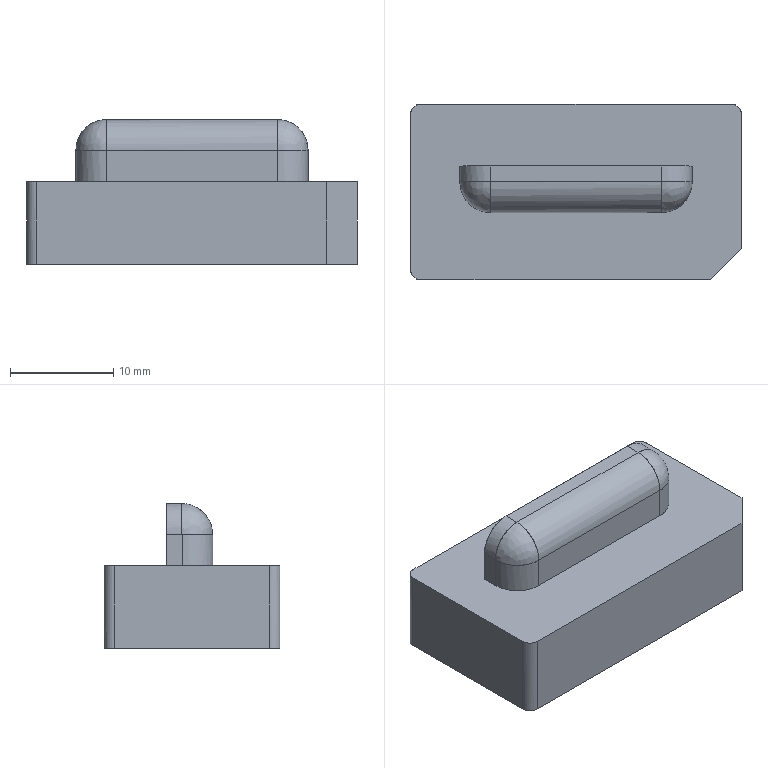NC program | PowerMill | posted with a generic post | part box 32 x 17 x 14 mm
Lines 1 to 1051 of 64476:
%
O0001
N104 ( POWERMILL CB  : 2026004.0)
N105 ( POST VER      : 2026.0.0.5161)
N106 ( OPTION FILE   : FANUC)
N107 ( OUTPUT WORKPLANE : WORLD)
N108 (  )
N109 ( TOOL LIST )
N110 (---------------------------------------)
N111 ( NO. | ID        | DIA.| TIP RAD|LENGTH)
N112 (---------------------------------------)
N113 (    1|D10C_1_1   |10.0 |  0.0   |69.44 )
N114 (    2|D4C_1_1    | 4.0 |  0.0   | 61.2 )
N115 (    3|D10_1_1    |10.0 |  0.0   |69.16 )
N116 (   22|R1.5_1_1   | 3.0 |  1.5   |59.88 )
N117 (   10|D3_1_1     | 3.0 |  0.0   |61.24 )
N118 (   13|TEXT_D4_1_1| 4.0 |  0.3   |61.24 )
N119 (---------------------------------------)
N120 (  )
N121 ( NUMBER OF TOOLPATHS: 10.0 )
N122 ( ESTIMATED PROGRAM DURATION: 0 HOURS 7 MIN 28 SEC)
N123 (  )
N124 G00 G21 G80 G40 G17
N125 G90
N126 G54
N127 G53 Z0.0
N128 (---------------)
N129 ( START TOOLPATH : 精公开粗01-扫面平行-D10C )
N130 (---------------)
N131 ( TOOL NO.    :1 )
N132 ( TOOL TYPE   : ENDMILL)
N133 ( TOOL ID     : D10C_1_1)
N134 ( TOOL DIA    : 10.0 LENGTH 69.44)
N135 T1
N136 M6
N137 S8000 M03
N138 G00 G90 X0.0 Y0.0
N139 G43 Z10.2 H1
N140
N141 G05 P10000 R4
N142 X23.78 Y11.28
N143 Z1.13
N144 G01 Z-0.07 F6000.0
N145 X18.78 F10000.0
N146 X-18.78
N147 Y5.64
N148 X18.78
N149 Y0.0
N150 X-18.78
N151 Y-5.64
N152 X18.78
N153 Y-11.28
N154 X-18.78
N155 X-23.78
N156 G00 Z10.2
N157 G05 P0
N158 (---------------)
N159 ( END TOOLPATH : 精公开粗01-扫面平行-D10C )
N160 (---------------)
N161 ( START TOOLPATH : 精公开粗01-外形偏置-D10C )
N162 (---------------)
N163 G00 X0.0 Y0.0 Z9.88
N164 G05 P10000 R4
N165 X-4.7475 Y16.555
N166 Z0.6873
N167 G01 Z-0.5127 F6000.0
N168 Y16.0275 F10000.0
N169 G03 X0.0 Y11.28 I4.7475 J0.0
N170 G01 X18.005
N171 G02 X19.005 Y10.28 I0.0 J-1.0
N172 G01 Y-10.28
N173 G02 X18.005 Y-11.28 I-1.0 J0.0
N174 G01 X-18.005
N175 G02 X-19.005 Y-10.28 I0.0 J1.0
N176 G01 Y10.28
N177 G02 X-18.005 Y11.28 I1.0 J0.0
N178 G01 X0.0
N179 Y7.7795
N180 X9.6678 Y7.7794
N181 X10.4413 Y7.7137
N182 X11.2147 Y7.5341
N183 X11.727 Y7.3476
N184 X11.9881 Y7.2269
N185 X12.7615 Y6.7642
N186 X13.0114 Y6.5741
N187 X13.535 Y6.0822
N188 X13.7827 Y5.8007
N189 X14.3008 Y5.0273
N190 X14.648 Y4.2538
N191 X14.8576 Y3.4804
N192 X14.946 Y2.707
N193 X14.9623 Y1.1601
N194 X14.9291 Y0.3867
N195 X14.8064 Y-0.3867
N196 X14.5826 Y-1.1601
N197 X14.3084 Y-1.8718
N198 X13.837 Y-2.707
N199 X13.535 Y-3.1226
N200 X13.2291 Y-3.4804
N201 X12.7615 Y-3.9525
N202 X11.9881 Y-4.5635
N203 X11.139 Y-5.0273
N204 X10.4413 Y-5.3345
N205 X9.6678 Y-5.5479
N206 X8.8944 Y-5.6648
N207 X8.121 Y-5.7014
N208 X7.3476 Y-5.6749
N209 X-7.3476
N210 X-8.121 Y-5.7014
N211 X-8.8944 Y-5.6648
N212 X-9.6678 Y-5.5479
N213 X-10.4413 Y-5.3345
N214 X-11.2147 Y-4.9948
N215 X-11.9881 Y-4.5635
N216 X-12.7615 Y-3.9525
N217 X-13.2281 Y-3.4804
N218 X-13.535 Y-3.1226
N219 X-13.8366 Y-2.707
N220 X-14.2792 Y-1.9336
N221 X-14.5833 Y-1.1601
N222 X-14.8064 Y-0.3867
N223 X-14.9293 Y0.3867
N224 X-14.9642 Y1.1601
N225 X-14.9379 Y1.9336
N226 X-14.938 Y1.9447
N227 X-14.946 Y2.707
N228 X-14.8576 Y3.4804
N229 X-14.6489 Y4.2538
N230 X-14.3084 Y5.0133
N231 X-13.7813 Y5.8007
N232 X-13.535 Y6.0822
N233 X-13.0105 Y6.5741
N234 X-12.7615 Y6.7643
N235 X-11.9881 Y7.2269
N236 X-11.727 Y7.3476
N237 X-11.2147 Y7.5341
N238 X-10.4413 Y7.7137
N239 X-9.6678 Y7.7795
N240 X0.0
N241 Y11.28
N242 G00 Z3.2947
N243 G01 X-4.7475 Y16.555
N244 G00 Z0.2947
N245 G01 Z-0.9053 F6000.0
N246 Y16.0275 F10000.0
N247 G03 X0.0 Y11.28 I4.7475 J0.0
N248 G01 X18.005
N249 G02 X19.005 Y10.28 I0.0 J-1.0
N250 G01 Y-10.28
N251 G02 X18.005 Y-11.28 I-1.0 J0.0
N252 G01 X-18.005
N253 G02 X-19.005 Y-10.28 I0.0 J1.0
N254 G01 Y10.28
N255 G02 X-18.005 Y11.28 I1.0 J0.0
N256 G01 X0.0
N257 Y7.7799
N258 X9.6678 Y7.78
N259 X10.4413 Y7.773
N260 X11.2147 Y7.6772
N261 X11.9881 Y7.4647
N262 X12.288 Y7.3476
N263 X12.7615 Y7.1167
N264 X13.535 Y6.5978
N265 X14.3323 Y5.8007
N266 X14.8503 Y5.0273
N267 X15.1967 Y4.2538
N268 X15.4058 Y3.4804
N269 X15.4941 Y2.707
N270 X15.5019 Y1.1601
N271 X15.477 Y0.3867
N272 X15.3697 Y-0.3867
N273 X15.1795 Y-1.1601
N274 X14.8776 Y-1.9336
N275 X14.3084 Y-2.9879
N276 X13.9629 Y-3.4804
N277 X13.535 Y-3.9652
N278 X12.7615 Y-4.6845
N279 X11.9881 Y-5.2139
N280 X11.2147 Y-5.6207
N281 X10.7558 Y-5.8007
N282 X9.6678 Y-6.1083
N283 X8.8944 Y-6.2143
N284 X8.121 Y-6.2473
N285 X7.3476 Y-6.2362
N286 X-7.3476
N287 X-7.3511
N288 X-8.121 Y-6.2473
N289 X-8.8944 Y-6.2143
N290 X-9.6678 Y-6.1083
N291 X-10.4413 Y-5.9009
N292 X-11.2147 Y-5.6207
N293 X-11.9881 Y-5.2139
N294 X-12.7615 Y-4.6845
N295 X-13.535 Y-3.9652
N296 X-13.962 Y-3.4804
N297 X-14.3084 Y-2.9879
N298 X-14.8775 Y-1.9336
N299 X-15.1782 Y-1.1601
N300 X-15.3701 Y-0.3867
N301 X-15.4765 Y0.3867
N302 X-15.5023 Y1.1601
N303 X-15.4941 Y2.707
N304 X-15.4058 Y3.4804
N305 X-15.1967 Y4.2538
N306 X-14.8495 Y5.0273
N307 X-14.3323 Y5.8007
N308 X-13.5644 Y6.5741
N309 X-12.7615 Y7.1167
N310 X-12.2881 Y7.3476
N311 X-11.9881 Y7.4647
N312 X-11.2147 Y7.6772
N313 X-10.4413 Y7.773
N314 X-9.6678 Y7.7799
N315 X0.0
N316 Y11.28
N317 G00 Z2.902
N318 G01 X-4.7475 Y16.555
N319 G00 Z-0.098
N320 G01 Z-1.298 F6000.0
N321 Y16.0275 F10000.0
N322 G03 X0.0 Y11.28 I4.7475 J0.0
N323 G01 X18.005
N324 G02 X19.005 Y10.28 I0.0 J-1.0
N325 G01 Y2.6987
N326 X15.8607 Y2.707
N327 X15.8552 Y0.6519
N328 X15.7409 Y-0.3867
N329 X15.5588 Y-1.1601
N330 X15.2753 Y-1.9336
N331 X14.9011 Y-2.707
N332 X14.4193 Y-3.4804
N333 X13.535 Y-4.4959
N334 X12.9128 Y-5.0273
N335 X11.9881 Y-5.643
N336 X11.2147 Y-6.0164
N337 X10.4413 Y-6.2931
N338 X9.6678 Y-6.4878
N339 X9.0419 Y-6.5741
N340 X8.121 Y-6.6169
N341 X7.3476 Y-6.6048
N342 X-7.3476
N343 X-7.3515 Y-6.6049
N344 X-8.121 Y-6.6169
N345 X-8.8944 Y-6.5868
N346 X-9.6678 Y-6.4878
N347 X-10.4413 Y-6.2931
N348 X-11.2147 Y-6.0164
N349 X-11.9881 Y-5.643
N350 X-12.7615 Y-5.1382
N351 X-13.535 Y-4.4959
N352 X-14.3084 Y-3.6271
N353 X-14.9011 Y-2.707
N354 X-15.2758 Y-1.9336
N355 X-15.559 Y-1.1601
N356 X-15.7409 Y-0.3867
N357 X-15.8552 Y0.6349
N358 X-15.8607 Y2.707
N359 X-15.7726 Y3.4804
N360 X-15.5638 Y4.2538
N361 X-15.2182 Y5.0273
N362 X-15.0818 Y5.2604
N363 X-14.7014 Y5.8007
N364 X-14.3084 Y6.2354
N365 X-13.9355 Y6.5741
N366 X-13.535 Y6.8718
N367 X-12.7615 Y7.3043
N368 X-11.9881 Y7.5844
N369 X-11.2147 Y7.7394
N370 X-10.4413 Y7.78
N371 X10.4413
N372 X11.2147 Y7.7394
N373 X11.9881 Y7.5844
N374 X12.6636 Y7.3476
N375 X13.535 Y6.8718
N376 X13.9355 Y6.5741
N377 X14.3084 Y6.2354
N378 X14.7014 Y5.8007
N379 X15.0818 Y5.2604
N380 X15.2182 Y5.0273
N381 X15.5638 Y4.2538
N382 X15.7726 Y3.4804
N383 X15.8607 Y2.707
N384 X19.005 Y2.6987
N385 Y-10.28
N386 G02 X18.005 Y-11.28 I-1.0 J0.0
N387 G01 X-18.005
N388 G02 X-19.005 Y-10.28 I0.0 J1.0
N389 G01 Y10.28
N390 G02 X-18.005 Y11.28 I1.0 J0.0
N391 G01 X0.0
N392 G00 Z2.5093
N393 G01 X-4.7475 Y16.555
N394 G00 Z-0.4907
N395 G01 Z-1.6907 F6000.0
N396 Y16.0275 F10000.0
N397 G03 X0.0 Y11.28 I4.7475 J0.0
N398 G01 X18.005
N399 G02 X19.005 Y10.28 I0.0 J-1.0
N400 G01 Y2.7264
N401 X16.1171 Y2.707
N402 X16.1275 Y1.1601
N403 X16.0988 Y0.3867
N404 X16.002 Y-0.3867
N405 X15.8552 Y-1.0664
N406 X15.5561 Y-1.9336
N407 X15.2037 Y-2.707
N408 X14.7313 Y-3.4804
N409 X14.13 Y-4.2538
N410 X13.535 Y-4.8475
N411 X12.7615 Y-5.4651
N412 X11.9881 Y-5.9427
N413 X11.2147 Y-6.2988
N414 X10.4378 Y-6.5741
N415 X9.6678 Y-6.7572
N416 X8.8944 Y-6.8524
N417 X8.121 Y-6.8816
N418 X7.3476 Y-6.8691
N419 X7.3435
N420 X-7.3476
N421 X-8.121 Y-6.8816
N422 X-8.8944 Y-6.8522
N423 X-9.6678 Y-6.7572
N424 X-10.4413 Y-6.5737
N425 X-11.2147 Y-6.2988
N426 X-11.9881 Y-5.9427
N427 X-12.7615 Y-5.4651
N428 X-13.3315 Y-5.0273
N429 X-14.1292 Y-4.2538
N430 X-14.7309 Y-3.4804
N431 X-15.0818 Y-2.9346
N432 X-15.5561 Y-1.9336
N433 X-15.8281 Y-1.1601
N434 X-16.0013 Y-0.3867
N435 X-16.0989 Y0.3867
N436 X-16.1274 Y1.1601
N437 X-16.118 Y2.707
N438 X-16.0298 Y3.4804
N439 X-15.8552 Y4.1544
N440 X-15.4772 Y5.0273
N441 X-14.9613 Y5.8007
N442 X-14.3084 Y6.4792
N443 X-13.535 Y7.0378
N444 X-12.9272 Y7.3476
N445 X-11.9881 Y7.6518
N446 X-11.2147 Y7.7647
N447 X-10.4413 Y7.78
N448 X10.4413
N449 X11.2147 Y7.7647
N450 X11.9881 Y7.6518
N451 X12.7615 Y7.4156
N452 X13.535 Y7.0378
N453 X14.1962 Y6.5741
N454 X14.9605 Y5.8007
N455 X15.4765 Y5.0273
N456 X15.8213 Y4.2538
N457 X16.03 Y3.4804
N458 X16.1171 Y2.707
N459 X19.005 Y2.7264
N460 Y-10.28
N461 G02 X18.005 Y-11.28 I-1.0 J0.0
N462 G01 X-18.005
N463 G02 X-19.005 Y-10.28 I0.0 J1.0
N464 G01 Y10.28
N465 G02 X-18.005 Y11.28 I1.0 J0.0
N466 G01 X0.0
N467 G00 Z2.1167
N468 G01 X-4.7475 Y16.555
N469 G00 Z-0.8833
N470 G01 Z-2.0833 F6000.0
N471 Y16.0275 F10000.0
N472 G03 X0.0 Y11.28 I4.7475 J0.0
N473 G01 X18.005
N474 G02 X19.005 Y10.28 I0.0 J-1.0
N475 G01 Y2.7189
N476 X16.3 Y2.707
N477 X16.3068 Y1.1601
N478 X16.2813 Y0.3867
N479 X16.1893 Y-0.3867
N480 X16.0132 Y-1.1601
N481 X15.757 Y-1.9336
N482 X15.411 Y-2.707
N483 X14.9567 Y-3.4804
N484 X14.366 Y-4.2538
N485 X13.6154 Y-5.0273
N486 X12.7615 Y-5.6928
N487 X11.9881 Y-6.1524
N488 X11.0276 Y-6.5741
N489 X10.4413 Y-6.7706
N490 X9.6678 Y-6.9453
N491 X8.8944 Y-7.0385
N492 X8.121 Y-7.0659
N493 X-8.121
N494 X-8.8944 Y-7.0385
N495 X-9.6678 Y-6.9453
N496 X-10.4413 Y-6.7706
N497 X-11.0267 Y-6.5741
N498 X-11.9881 Y-6.1524
N499 X-12.7615 Y-5.6928
N500 X-13.535 Y-5.0949
N501 X-14.3084 Y-4.3232
N502 X-14.9569 Y-3.4804
N503 X-15.411 Y-2.707
N504 X-15.7574 Y-1.9336
N505 X-16.0131 Y-1.1601
N506 X-16.1898 Y-0.3867
N507 X-16.2812 Y0.3867
N508 X-16.3071 Y1.1601
N509 X-16.2996 Y2.707
N510 X-16.2129 Y3.4804
N511 X-16.0037 Y4.2538
N512 X-15.8552 Y4.63
N513 X-15.6598 Y5.0273
N514 X-15.145 Y5.8007
N515 X-14.381 Y6.5741
N516 X-13.535 Y7.1447
N517 X-13.1143 Y7.3476
N518 X-12.7615 Y7.4858
N519 X-11.9881 Y7.6901
N520 X-11.2147 Y7.7749
N521 X-10.4413 Y7.78
N522 X10.4413
N523 X11.2147 Y7.7749
N524 X11.9881 Y7.6901
N525 X12.7615 Y7.4858
N526 X13.1143 Y7.3476
N527 X13.535 Y7.1447
N528 X14.3084 Y6.6328
N529 X15.0818 Y5.8769
N530 X15.6591 Y5.0273
N531 X15.8552 Y4.63
N532 X16.0043 Y4.2538
N533 X16.2118 Y3.4804
N534 X16.3 Y2.707
N535 X19.005 Y2.7189
N536 Y-10.28
N537 G02 X18.005 Y-11.28 I-1.0 J0.0
N538 G01 X-18.005
N539 G02 X-19.005 Y-10.28 I0.0 J1.0
N540 G01 Y10.28
N541 G02 X-18.005 Y11.28 I1.0 J0.0
N542 G01 X0.0
N543 G00 Z1.724
N544 G01 X-4.7475 Y16.555
N545 G00 Z-1.276
N546 G01 Z-2.476 F6000.0
N547 Y16.0275 F10000.0
N548 G03 X0.0 Y11.28 I4.7475 J0.0
N549 G01 X18.005
N550 G02 X19.005 Y10.28 I0.0 J-1.0
N551 G01 Y2.7158
N552 X16.4188 Y2.707
N553 X16.424 Y1.1601
N554 X16.4017 Y0.3867
N555 X16.3114 Y-0.3867
N556 X16.1349 Y-1.1601
N557 X15.8923 Y-1.9336
N558 X15.5464 Y-2.707
N559 X15.0985 Y-3.4804
N560 X14.5384 Y-4.2538
N561 X13.8012 Y-5.0273
N562 X13.535 Y-5.2601
N563 X12.8238 Y-5.8007
N564 X11.9881 Y-6.2908
N565 X11.3798 Y-6.5741
N566 X10.4413 Y-6.9003
N567 X9.6678 Y-7.0696
N568 X8.8944 Y-7.162
N569 X8.121 Y-7.1891
N570 X7.3476 Y-7.1839
N571 X-7.3476
N572 X-7.3492
N573 X-8.121 Y-7.1891
N574 X-8.8944 Y-7.1617
N575 X-9.6678 Y-7.0696
N576 X-10.4413 Y-6.9003
N577 X-11.2147 Y-6.6354
N578 X-11.9881 Y-6.2908
N579 X-12.7615 Y-5.8428
N580 X-13.535 Y-5.2601
N581 X-13.8013 Y-5.0273
N582 X-14.5382 Y-4.2538
N583 X-15.0818 Y-3.5051
N584 X-15.5465 Y-2.707
N585 X-15.8552 Y-2.0257
N586 X-16.1351 Y-1.1601
N587 X-16.3121 Y-0.3867
N588 X-16.402 Y0.3867
N589 X-16.4238 Y1.1601
N590 X-16.4201 Y2.707
N591 X-16.331 Y3.4804
N592 X-16.1237 Y4.2538
N593 X-15.8552 Y4.8823
N594 X-15.2634 Y5.8007
N595 X-15.0818 Y6.0155
N596 X-14.5011 Y6.5741
N597 X-14.3084 Y6.7263
N598 X-13.535 Y7.2065
N599 X-13.2348 Y7.3476
N600 X-12.7615 Y7.5253
N601 X-11.9881 Y7.7116
N602 X-11.2147 Y7.7793
N603 X-10.5421
N604 X-10.4413 Y7.7799
N605 X10.4413
N606 X10.5421 Y7.7793
N607 X11.2147
N608 X11.9881 Y7.7116
N609 X12.7615 Y7.5253
N610 X13.2345 Y7.3476
N611 X13.535 Y7.2065
N612 X14.3084 Y6.7263
N613 X14.5005 Y6.5741
N614 X15.0818 Y6.0155
N615 X15.2632 Y5.8007
N616 X15.7782 Y5.0273
N617 X16.1229 Y4.2538
N618 X16.3309 Y3.4804
N619 X16.4188 Y2.707
N620 X19.005 Y2.7158
N621 Y-10.28
N622 G02 X18.005 Y-11.28 I-1.0 J0.0
N623 G01 X-18.005
N624 G02 X-19.005 Y-10.28 I0.0 J1.0
N625 G01 Y10.28
N626 G02 X-18.005 Y11.28 I1.0 J0.0
N627 G01 X0.0
N628 G00 Z1.3313
N629 G01 X-4.7475 Y16.555
N630 G00 Z-1.6687
N631 G01 Z-2.8687 F6000.0
N632 Y16.0275 F10000.0
N633 G03 X0.0 Y11.28 I4.7475 J0.0
N634 G01 X18.005
N635 G02 X19.005 Y10.28 I0.0 J-1.0
N636 G01 Y2.6928
N637 X16.4814 Y2.707
N638 X16.4684 Y0.3867
N639 X16.3715 Y-0.3867
N640 X16.2123 Y-1.1601
N641 X15.8552 Y-2.2105
N642 X15.6204 Y-2.707
N643 X15.1876 Y-3.4804
N644 X14.6251 Y-4.2538
N645 X13.8992 Y-5.0273
N646 X13.535 Y-5.3536
N647 X12.7615 Y-5.9274
N648 X11.9881 Y-6.3666
N649 X11.565 Y-6.5741
N650 X10.4413 Y-6.968
N651 X9.6678 Y-7.1362
N652 X8.8944 Y-7.2307
N653 X8.121 Y-7.2576
N654 X7.3476 Y-7.2477
N655 X-7.3476
N656 X-7.3507 Y-7.2478
N657 X-8.121 Y-7.2576
N658 X-8.8944 Y-7.2302
N659 X-9.6678 Y-7.1362
N660 X-10.4413 Y-6.968
N661 X-11.5604 Y-6.5741
N662 X-11.9881 Y-6.3666
N663 X-12.7615 Y-5.9274
N664 X-13.535 Y-5.3536
N665 X-13.8991 Y-5.0273
N666 X-14.6249 Y-4.2538
N667 X-15.0818 Y-3.6353
N668 X-15.6208 Y-2.707
N669 X-15.8552 Y-2.2105
N670 X-16.2122 Y-1.1601
N671 X-16.3715 Y-0.3867
N672 X-16.4698 Y0.3867
N673 X-16.4814 Y2.707
N674 X-16.3937 Y3.4804
N675 X-16.1857 Y4.2538
N676 X-15.8413 Y5.0273
N677 X-15.3265 Y5.8007
N678 X-15.0818 Y6.085
N679 X-14.564 Y6.5741
N680 X-14.3084 Y6.7719
N681 X-13.535 Y7.2383
N682 X-12.7615 Y7.5454
N683 X-11.9881 Y7.7207
N684 X-11.2147 Y7.7799
N685 X11.2147
N686 X11.9881 Y7.7207
N687 X12.7615 Y7.5454
N688 X13.535 Y7.2383
N689 X14.3084 Y6.7719
N690 X14.564 Y6.5741
N691 X15.0818 Y6.085
N692 X15.3266 Y5.8007
N693 X15.8413 Y5.0273
N694 X16.1857 Y4.2538
N695 X16.3936 Y3.4804
N696 X16.4814 Y2.707
N697 X19.005 Y2.6928
N698 Y-10.28
N699 G02 X18.005 Y-11.28 I-1.0 J0.0
N700 G01 X-18.005
N701 G02 X-19.005 Y-10.28 I0.0 J1.0
N702 G01 Y10.28
N703 G02 X-18.005 Y11.28 I1.0 J0.0
N704 G01 X0.0
N705 G00 Z0.9387
N706 G01 X-4.7475 Y16.555
N707 G00 Z-2.0613
N708 G01 Z-3.2613 F6000.0
N709 Y16.0275 F10000.0
N710 G03 X0.0 Y11.28 I4.7475 J0.0
N711 G01 X18.005
N712 G02 X19.005 Y10.28 I0.0 J-1.0
N713 G01 Y2.7136
N714 X16.5017 Y2.707
N715 X16.5057 Y1.1601
N716 X16.48 Y0.3867
N717 X16.3964 Y-0.3867
N718 X16.2304 Y-1.1601
N719 X15.9824 Y-1.9336
N720 X15.6447 Y-2.707
N721 X15.2112 Y-3.4804
N722 X14.6515 Y-4.2538
N723 X13.9304 Y-5.0273
N724 X13.535 Y-5.3804
N725 X12.7615 Y-5.9496
N726 X11.9881 Y-6.3913
N727 X11.6104 Y-6.5741
N728 X11.2147 Y-6.7354
N729 X10.4413 Y-6.9899
N730 X9.6678 Y-7.1612
N731 X8.8944 Y-7.2506
N732 X8.121 Y-7.2799
N733 X-8.121
N734 X-8.8944 Y-7.2506
N735 X-9.6678 Y-7.1612
N736 X-10.4413 Y-6.9899
N737 X-11.2147 Y-6.7354
N738 X-11.9881 Y-6.3913
N739 X-12.7615 Y-5.9496
N740 X-13.535 Y-5.3804
N741 X-13.9304 Y-5.0273
N742 X-14.6515 Y-4.2538
N743 X-15.0818 Y-3.6768
N744 X-15.6447 Y-2.707
N745 X-15.9825 Y-1.9336
N746 X-16.2303 Y-1.1601
N747 X-16.3964 Y-0.3867
N748 X-16.48 Y0.3867
N749 X-16.5058 Y1.1601
N750 X-16.5017 Y2.707
N751 X-16.4139 Y3.4804
N752 X-16.2059 Y4.2538
N753 X-15.8616 Y5.0273
N754 X-15.3469 Y5.8007
N755 X-15.0818 Y6.1067
N756 X-14.5843 Y6.5741
N757 X-14.3084 Y6.7867
N758 X-13.535 Y7.2483
N759 X-12.7615 Y7.5516
N760 X-11.9881 Y7.7246
N761 X-11.2147 Y7.7799
N762 X11.2147
N763 X11.9881 Y7.7246
N764 X12.7615 Y7.5516
N765 X13.535 Y7.2483
N766 X14.3084 Y6.7867
N767 X14.5843 Y6.5741
N768 X15.0818 Y6.1067
N769 X15.3468 Y5.8007
N770 X15.8552 Y5.039
N771 X16.2059 Y4.2538
N772 X16.4139 Y3.4804
N773 X16.5017 Y2.707
N774 X19.005 Y2.7136
N775 Y-10.28
N776 G02 X18.005 Y-11.28 I-1.0 J0.0
N777 G01 X-18.005
N778 G02 X-19.005 Y-10.28 I0.0 J1.0
N779 G01 Y10.28
N780 G02 X-18.005 Y11.28 I1.0 J0.0
N781 G01 X0.0
N782 G00 Z0.546
N783 G01 X-4.7475 Y16.555
N784 G00 Z-2.454
N785 G01 Z-3.654 F6000.0
N786 Y16.0275 F10000.0
N787 G03 X0.0 Y11.28 I4.7475 J0.0
N788 G01 X18.005
N789 G02 X19.005 Y10.28 I0.0 J-1.0
N790 G01 Y2.7136
N791 X16.5017 Y2.707
N792 X16.5058 Y1.1601
N793 X16.48 Y0.3867
N794 X16.3965 Y-0.3867
N795 X16.2304 Y-1.1601
N796 X15.9824 Y-1.9336
N797 X15.6447 Y-2.707
N798 X15.2112 Y-3.4804
N799 X14.6515 Y-4.2538
N800 X13.9305 Y-5.0273
N801 X13.535 Y-5.3804
N802 X12.7615 Y-5.9496
N803 X11.9881 Y-6.3913
N804 X11.6104 Y-6.5741
N805 X11.2147 Y-6.7355
N806 X10.4413 Y-6.9899
N807 X9.6678 Y-7.1612
N808 X8.8944 Y-7.2506
N809 X8.121 Y-7.2799
N810 X-8.121
N811 X-8.8944 Y-7.2506
N812 X-9.6678 Y-7.1612
N813 X-10.4413 Y-6.9899
N814 X-11.2147 Y-6.7355
N815 X-11.9881 Y-6.3913
N816 X-12.7615 Y-5.9496
N817 X-13.535 Y-5.3804
N818 X-13.9304 Y-5.0273
N819 X-14.6515 Y-4.2538
N820 X-15.0818 Y-3.6768
N821 X-15.6447 Y-2.707
N822 X-15.9825 Y-1.9336
N823 X-16.2304 Y-1.1601
N824 X-16.3964 Y-0.3867
N825 X-16.48 Y0.3867
N826 X-16.5058 Y1.1601
N827 X-16.5017 Y2.707
N828 X-16.4139 Y3.4804
N829 X-16.2059 Y4.2538
N830 X-15.8616 Y5.0273
N831 X-15.3469 Y5.8007
N832 X-15.0818 Y6.1067
N833 X-14.5843 Y6.5741
N834 X-14.3084 Y6.7867
N835 X-13.535 Y7.2483
N836 X-12.7615 Y7.5516
N837 X-11.9881 Y7.7246
N838 X-11.2147 Y7.7799
N839 X11.2147
N840 X11.9881 Y7.7246
N841 X12.7615 Y7.5516
N842 X13.535 Y7.2483
N843 X14.3084 Y6.7867
N844 X14.5843 Y6.5741
N845 X15.0818 Y6.1067
N846 X15.3468 Y5.8007
N847 X15.8552 Y5.039
N848 X16.2059 Y4.2538
N849 X16.4139 Y3.4804
N850 X16.5017 Y2.707
N851 X19.005 Y2.7136
N852 Y-10.28
N853 G02 X18.005 Y-11.28 I-1.0 J0.0
N854 G01 X-18.005
N855 G02 X-19.005 Y-10.28 I0.0 J1.0
N856 G01 Y10.28
N857 G02 X-18.005 Y11.28 I1.0 J0.0
N858 G01 X0.0
N859 G00 Z0.1533
N860 G01 X-4.7475 Y16.555
N861 G00 Z-2.8467
N862 G01 Z-4.0467 F6000.0
N863 Y16.0275 F10000.0
N864 G03 X0.0 Y11.28 I4.7475 J0.0
N865 G01 X18.005
N866 G02 X19.005 Y10.28 I0.0 J-1.0
N867 G01 Y2.7136
N868 X16.5017 Y2.707
N869 X16.5058 Y1.1601
N870 X16.48 Y0.3867
N871 X16.3965 Y-0.3867
N872 X16.2304 Y-1.1601
N873 X15.9825 Y-1.9336
N874 X15.6448 Y-2.707
N875 X15.2113 Y-3.4804
N876 X14.6515 Y-4.2538
N877 X13.9305 Y-5.0273
N878 X13.535 Y-5.3804
N879 X12.7615 Y-5.9497
N880 X11.9881 Y-6.3913
N881 X11.6104 Y-6.5741
N882 X11.2147 Y-6.7355
N883 X10.4413 Y-6.9899
N884 X9.6678 Y-7.1612
N885 X8.8944 Y-7.2506
N886 X8.121 Y-7.2799
N887 X-8.121
N888 X-8.8944 Y-7.2506
N889 X-9.6678 Y-7.1612
N890 X-10.4413 Y-6.9899
N891 X-11.2147 Y-6.7355
N892 X-11.9881 Y-6.3913
N893 X-12.7615 Y-5.9497
N894 X-13.535 Y-5.3804
N895 X-13.9305 Y-5.0273
N896 X-14.6515 Y-4.2538
N897 X-15.0818 Y-3.6769
N898 X-15.6447 Y-2.707
N899 X-15.9825 Y-1.9336
N900 X-16.2304 Y-1.1601
N901 X-16.3965 Y-0.3867
N902 X-16.48 Y0.3867
N903 X-16.5058 Y1.1601
N904 X-16.5017 Y2.707
N905 X-16.4139 Y3.4804
N906 X-16.2059 Y4.2538
N907 X-15.8616 Y5.0273
N908 X-15.3469 Y5.8007
N909 X-15.0818 Y6.1068
N910 X-14.5843 Y6.5741
N911 X-14.3084 Y6.7867
N912 X-13.535 Y7.2483
N913 X-12.7615 Y7.5516
N914 X-11.9881 Y7.7246
N915 X-11.2147 Y7.78
N916 X11.2147
N917 X11.9881 Y7.7246
N918 X12.7615 Y7.5516
N919 X13.535 Y7.2483
N920 X14.3084 Y6.7867
N921 X14.5843 Y6.5741
N922 X15.0818 Y6.1068
N923 X15.3468 Y5.8007
N924 X15.8552 Y5.039
N925 X16.2059 Y4.2538
N926 X16.414 Y3.4804
N927 X16.5017 Y2.707
N928 X19.005 Y2.7136
N929 Y-10.28
N930 G02 X18.005 Y-11.28 I-1.0 J0.0
N931 G01 X-18.005
N932 G02 X-19.005 Y-10.28 I0.0 J1.0
N933 G01 Y10.28
N934 G02 X-18.005 Y11.28 I1.0 J0.0
N935 G01 X0.0
N936 G00 Z-0.2393
N937 G01 X-4.7475 Y16.555
N938 G00 Z-3.2393
N939 G01 Z-4.4393 F6000.0
N940 Y16.0275 F10000.0
N941 G03 X0.0 Y11.28 I4.7475 J0.0
N942 G01 X18.005
N943 G02 X19.005 Y10.28 I0.0 J-1.0
N944 G01 Y2.7136
N945 X16.5017 Y2.707
N946 X16.5058 Y1.1601
N947 X16.48 Y0.3867
N948 X16.3965 Y-0.3867
N949 X16.2304 Y-1.1601
N950 X15.9825 Y-1.9336
N951 X15.6448 Y-2.707
N952 X15.2113 Y-3.4804
N953 X14.6515 Y-4.2538
N954 X13.9305 Y-5.0273
N955 X13.535 Y-5.3804
N956 X12.7615 Y-5.9497
N957 X11.9881 Y-6.3914
N958 X11.6104 Y-6.5741
N959 X11.2147 Y-6.7355
N960 X10.4413 Y-6.9899
N961 X9.6678 Y-7.1612
N962 X8.8944 Y-7.2506
N963 X8.121 Y-7.28
N964 X-8.121
N965 X-8.8944 Y-7.2506
N966 X-9.6678 Y-7.1612
N967 X-10.4413 Y-6.9899
N968 X-11.2147 Y-6.7355
N969 X-11.9881 Y-6.3914
N970 X-12.7615 Y-5.9497
N971 X-13.535 Y-5.3804
N972 X-13.9305 Y-5.0273
N973 X-14.6515 Y-4.2538
N974 X-15.0818 Y-3.6769
N975 X-15.6447 Y-2.707
N976 X-15.9825 Y-1.9336
N977 X-16.2304 Y-1.1601
N978 X-16.3965 Y-0.3867
N979 X-16.48 Y0.3867
N980 X-16.5058 Y1.1601
N981 X-16.5017 Y2.707
N982 X-16.4139 Y3.4804
N983 X-16.2059 Y4.2538
N984 X-15.8616 Y5.0273
N985 X-15.3469 Y5.8007
N986 X-15.0818 Y6.1068
N987 X-14.5843 Y6.5741
N988 X-14.3084 Y6.7868
N989 X-13.535 Y7.2483
N990 X-12.7615 Y7.5517
N991 X-11.9881 Y7.7247
N992 X-11.2147 Y7.78
N993 X11.2147
N994 X11.9881 Y7.7247
N995 X12.7615 Y7.5517
N996 X13.535 Y7.2483
N997 X14.3084 Y6.7868
N998 X14.5843 Y6.5741
N999 X15.0818 Y6.1068
N1000 X15.3469 Y5.8007
N1001 X15.8552 Y5.039
N1002 X16.2059 Y4.2538
N1003 X16.414 Y3.4804
N1004 X16.5017 Y2.707
N1005 X19.005 Y2.7136
N1006 Y-10.28
N1007 G02 X18.005 Y-11.28 I-1.0 J0.0
N1008 G01 X-18.005
N1009 G02 X-19.005 Y-10.28 I0.0 J1.0
N1010 G01 Y10.28
N1011 G02 X-18.005 Y11.28 I1.0 J0.0
N1012 G01 X0.0
N1013 G00 Z-0.632
N1014 G01 X-4.7475 Y16.555
N1015 G00 Z-3.632
N1016 G01 Z-4.832 F6000.0
N1017 Y16.0275 F10000.0
N1018 G03 X0.0 Y11.28 I4.7475 J0.0
N1019 G01 X18.005
N1020 G02 X19.005 Y10.28 I0.0 J-1.0
N1021 G01 Y2.7136
N1022 X16.5017 Y2.707
N1023 X16.5058 Y1.1601
N1024 X16.48 Y0.3867
N1025 X16.3965 Y-0.3867
N1026 X16.2304 Y-1.1601
N1027 X15.9825 Y-1.9336
N1028 X15.6448 Y-2.707
N1029 X15.2113 Y-3.4804
N1030 X14.6515 Y-4.2538
N1031 X13.9305 Y-5.0273
N1032 X13.535 Y-5.3804
N1033 X12.7615 Y-5.9497
N1034 X11.9881 Y-6.3914
N1035 X11.6105 Y-6.5741
N1036 X11.2147 Y-6.7355
N1037 X10.4413 Y-6.9899
N1038 X9.6678 Y-7.1612
N1039 X8.8944 Y-7.2506
N1040 X8.121 Y-7.28
N1041 X-8.121
N1042 X-8.8944 Y-7.2506
N1043 X-9.6678 Y-7.1612
N1044 X-10.4413 Y-6.9899
N1045 X-11.2147 Y-6.7355
N1046 X-11.9881 Y-6.3914
N1047 X-12.7615 Y-5.9497
N1048 X-13.535 Y-5.3804
N1049 X-13.9305 Y-5.0273
N1050 X-14.6515 Y-4.2538
N1051 X-15.0818 Y-3.6769
N1052 X-15.6448 Y-2.707
N1053 X-15.9825 Y-1.9336
N1054 X-16.2304 Y-1.1601
N1055 X-16.3965 Y-0.3867
N1056 X-16.4801 Y0.3867
N1057 X-16.5058 Y1.1601
N1058 X-16.5017 Y2.707
N1059 X-16.4139 Y3.4804
N1060 X-16.2059 Y4.2538
N1061 X-15.8616 Y5.0273
N1062 X-15.347 Y5.8007
N1063 X-15.0818 Y6.1068
N1064 X-14.5843 Y6.5741
N1065 X-14.3084 Y6.7868
N1066 X-13.535 Y7.2483
N1067 X-12.7615 Y7.5517
N1068 X-11.9881 Y7.7247
N1069 X-11.2147 Y7.78
N1070 X11.2147
N1071 X11.9881 Y7.7247
N1072 X12.7615 Y7.5517
N1073 X13.535 Y7.2483
N1074 X14.3084 Y6.7868
N1075 X14.5844 Y6.5741
N1076 X15.0818 Y6.1068
N1077 X15.3469 Y5.8007
N1078 X15.8552 Y5.039
N1079 X16.2059 Y4.2538
N1080 X16.414 Y3.4804
N1081 X16.5017 Y2.707
N1082 X19.005 Y2.7136
N1083 Y-10.28
N1084 G02 X18.005 Y-11.28 I-1.0 J0.0
N1085 G01 X-18.005
N1086 G02 X-19.005 Y-10.28 I0.0 J1.0
N1087 G01 Y10.28
N1088 G02 X-18.005 Y11.28 I1.0 J0.0
N1089 G01 X0.0
N1090 G00 Z-1.0247
N1091 G01 X-4.7475 Y16.555
N1092 G00 Z-4.0247
N1093 G01 Z-5.2247 F6000.0
N1094 Y16.0275 F10000.0
N1095 G03 X0.0 Y11.28 I4.7475 J0.0
N1096 G01 X18.005
N1097 G02 X19.005 Y10.28 I0.0 J-1.0
N1098 G01 Y2.7136
N1099 X16.5018 Y2.707
N1100 X16.5058 Y1.1601
N1101 X16.48 Y0.3867
N1102 X16.3965 Y-0.3867
N1103 X16.2305 Y-1.1601
N1104 X15.9825 Y-1.9336
N1105 X15.6448 Y-2.707
N1106 X15.2113 Y-3.4804
N1107 X14.6515 Y-4.2538
N1108 X13.9305 Y-5.0273
N1109 X13.535 Y-5.3804
N1110 X12.7615 Y-5.9497
N1111 X11.9881 Y-6.3914
N1112 X11.6105 Y-6.5741
N1113 X11.2147 Y-6.7355
N1114 X10.4413 Y-6.9899
N1115 X9.6678 Y-7.1613
N1116 X8.8944 Y-7.2507
N1117 X8.121 Y-7.28
N1118 X-8.121
N1119 X-8.8944 Y-7.2507
N1120 X-9.6678 Y-7.1613
N1121 X-10.4413 Y-6.9899
N1122 X-11.2147 Y-6.7355
N1123 X-11.9881 Y-6.3914
N1124 X-12.7615 Y-5.9497
N1125 X-13.535 Y-5.3804
N1126 X-13.9305 Y-5.0273
N1127 X-14.6515 Y-4.2538
N1128 X-15.0818 Y-3.6769
N1129 X-15.6448 Y-2.707
N1130 X-15.9825 Y-1.9336
N1131 X-16.2304 Y-1.1601
N1132 X-16.3965 Y-0.3867
N1133 X-16.4801 Y0.3867
N1134 X-16.5058 Y1.1601
N1135 X-16.5018 Y2.707
N1136 X-16.4139 Y3.4804
N1137 X-16.206 Y4.2538
N1138 X-15.8616 Y5.0273
N1139 X-15.347 Y5.8007
N1140 X-15.0818 Y6.1068
N1141 X-14.5843 Y6.5741
N1142 X-14.3084 Y6.7868
N1143 X-13.535 Y7.2483
N1144 X-12.7615 Y7.5517
N1145 X-11.9881 Y7.7247
N1146 X-11.2147 Y7.78
N1147 X11.2147
N1148 X11.9881 Y7.7247